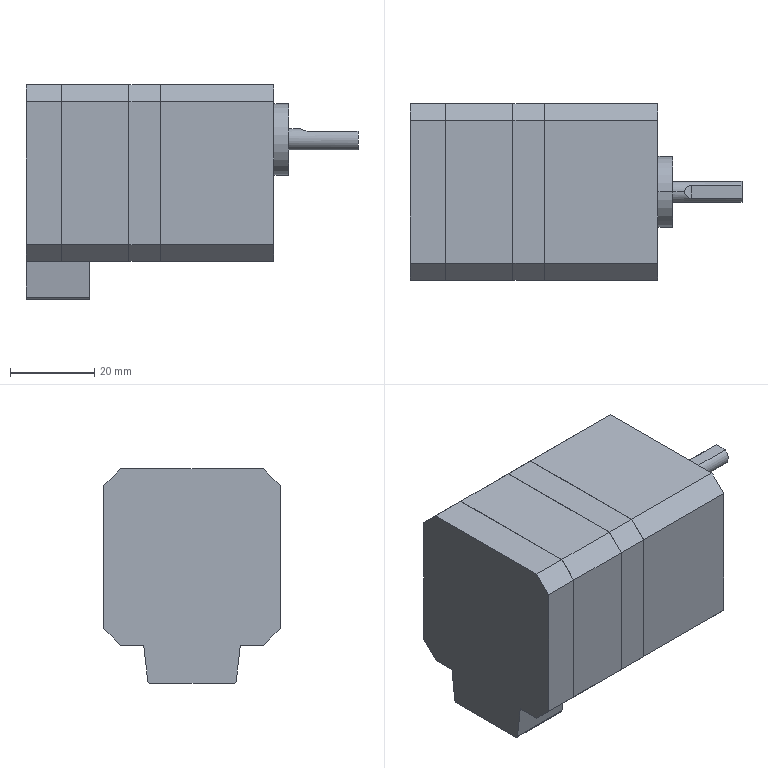Part | SolidWorks | features ICE 8, Chamfer 1, Extrusion 1, Fillet 1, HoleWzd 1, Revolution 1 | 1 solid | 122 faces | box 79 x 42 x 51 mm | volume 105451 mm3 | plane 85 | cylinder 29 | cone 8 | commonest cylinder face diameters 1 x14 2.5 x8 5 x2 17 x2 38 x2 6 x1